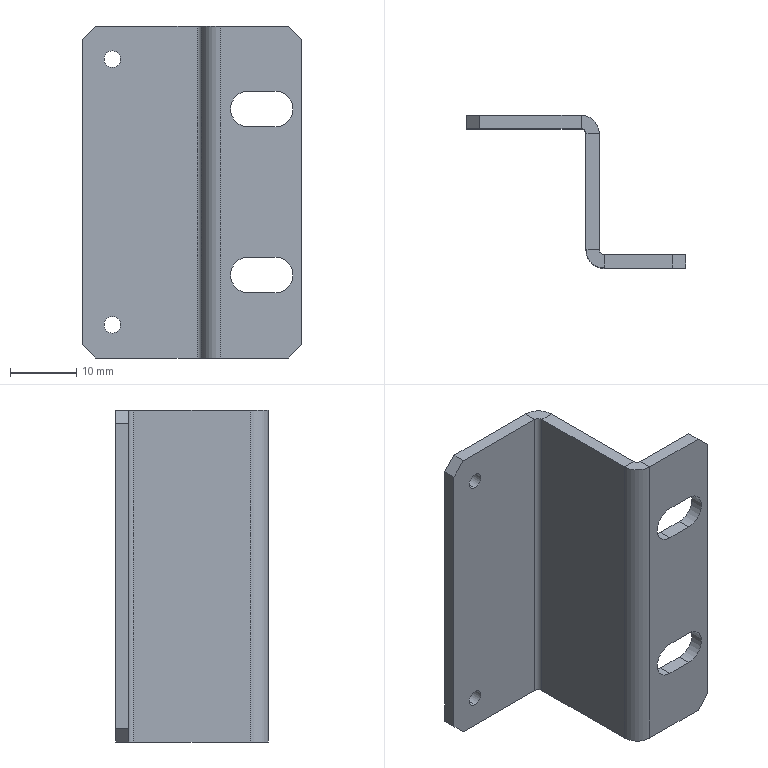Part | STEP file | 11-GYZB-JJ-00511 | 1 solid | 38 faces | box 33 x 23 x 50 mm | volume 5037 mm3 | plane 26 | cylinder 12 | commonest cylinder face diameters 2.5 x4 5.4 x4 1.473 x2 5.473 x2
STEP:
#1=CARTESIAN_POINT('',(-13.5,21.,-21.25));
#2=VERTEX_POINT('',#1);
#3=CARTESIAN_POINT('',(-13.5,21.,-18.75));
#4=VERTEX_POINT('',#3);
#5=CARTESIAN_POINT('',(-13.5,21.,-20.));
#6=DIRECTION('',(0.,1.,0.));
#7=DIRECTION('',(-1.,0.,0.));
#8=AXIS2_PLACEMENT_3D('',#5,#6,#7);
#9=CIRCLE('',#8,1.25);
#10=EDGE_CURVE('',#2,#4,#9,.T.);
#11=ORIENTED_EDGE('',*,*,#10,.F.);
#12=CARTESIAN_POINT('',(-13.5,23.,-21.25));
#13=VERTEX_POINT('',#12);
#14=CARTESIAN_POINT('',(-13.5,23.,-21.25));
#15=DIRECTION('',(0.,1.,0.));
#16=VECTOR('',#15,1000.);
#17=LINE('',#14,#16);
#18=EDGE_CURVE('',#2,#13,#17,.T.);
#19=ORIENTED_EDGE('',*,*,#18,.T.);
#20=CARTESIAN_POINT('',(-13.5,23.,-18.75));
#21=VERTEX_POINT('',#20);
#22=CARTESIAN_POINT('',(-13.5,23.,-20.));
#23=DIRECTION('',(0.,1.,0.));
#24=DIRECTION('',(0.,0.,1.));
#25=AXIS2_PLACEMENT_3D('',#22,#23,#24);
#26=CIRCLE('',#25,1.25);
#27=EDGE_CURVE('',#13,#21,#26,.T.);
#28=ORIENTED_EDGE('',*,*,#27,.T.);
#29=CARTESIAN_POINT('',(-13.5,23.,-18.75));
#30=DIRECTION('',(0.,1.,0.));
#31=VECTOR('',#30,1000.);
#32=LINE('',#29,#31);
#33=EDGE_CURVE('',#4,#21,#32,.T.);
#34=ORIENTED_EDGE('',*,*,#33,.F.);
#35=EDGE_LOOP('',(#11,#19,#28,#34));
#36=FACE_OUTER_BOUND('',#35,.T.);
#37=CARTESIAN_POINT('',(-13.5,23.,-20.));
#38=DIRECTION('',(0.,1.,0.));
#39=DIRECTION('',(0.,0.,1.));
#40=AXIS2_PLACEMENT_3D('',#37,#38,#39);
#41=CYLINDRICAL_SURFACE('',#40,1.25);
#42=ADVANCED_FACE('',(#36),#41,.F.);
#43=CARTESIAN_POINT('',(-13.5,21.,18.75));
#44=VERTEX_POINT('',#43);
#45=CARTESIAN_POINT('',(-13.5,21.,21.25));
#46=VERTEX_POINT('',#45);
#47=CARTESIAN_POINT('',(-13.5,21.,20.));
#48=DIRECTION('',(0.,1.,0.));
#49=DIRECTION('',(-1.,0.,0.));
#50=AXIS2_PLACEMENT_3D('',#47,#48,#49);
#51=CIRCLE('',#50,1.25);
#52=EDGE_CURVE('',#44,#46,#51,.T.);
#53=ORIENTED_EDGE('',*,*,#52,.F.);
#54=CARTESIAN_POINT('',(-13.5,23.,18.75));
#55=VERTEX_POINT('',#54);
#56=CARTESIAN_POINT('',(-13.5,23.,18.75));
#57=DIRECTION('',(0.,1.,0.));
#58=VECTOR('',#57,1000.);
#59=LINE('',#56,#58);
#60=EDGE_CURVE('',#44,#55,#59,.T.);
#61=ORIENTED_EDGE('',*,*,#60,.T.);
#62=CARTESIAN_POINT('',(-13.5,23.,21.25));
#63=VERTEX_POINT('',#62);
#64=CARTESIAN_POINT('',(-13.5,23.,20.));
#65=DIRECTION('',(0.,1.,0.));
#66=DIRECTION('',(0.,0.,1.));
#67=AXIS2_PLACEMENT_3D('',#64,#65,#66);
#68=CIRCLE('',#67,1.25);
#69=EDGE_CURVE('',#55,#63,#68,.T.);
#70=ORIENTED_EDGE('',*,*,#69,.T.);
#71=CARTESIAN_POINT('',(-13.5,23.,21.25));
#72=DIRECTION('',(0.,1.,0.));
#73=VECTOR('',#72,1000.);
#74=LINE('',#71,#73);
#75=EDGE_CURVE('',#46,#63,#74,.T.);
#76=ORIENTED_EDGE('',*,*,#75,.F.);
#77=EDGE_LOOP('',(#53,#61,#70,#76));
#78=FACE_OUTER_BOUND('',#77,.T.);
#79=CARTESIAN_POINT('',(-13.5,23.,20.));
#80=DIRECTION('',(0.,1.,0.));
#81=DIRECTION('',(0.,0.,1.));
#82=AXIS2_PLACEMENT_3D('',#79,#80,#81);
#83=CYLINDRICAL_SURFACE('',#82,1.25);
#84=ADVANCED_FACE('',(#78),#83,.F.);
#85=CARTESIAN_POINT('',(2.,20.263,-25.));
#86=VERTEX_POINT('',#85);
#87=CARTESIAN_POINT('',(2.,2.737,-25.));
#88=VERTEX_POINT('',#87);
#89=CARTESIAN_POINT('',(2.,0.,-25.));
#90=DIRECTION('',(0.,-1.,0.));
#91=VECTOR('',#90,1000.);
#92=LINE('',#89,#91);
#93=EDGE_CURVE('',#86,#88,#92,.T.);
#94=ORIENTED_EDGE('',*,*,#93,.F.);
#95=CARTESIAN_POINT('',(2.,20.263,25.));
#96=VERTEX_POINT('',#95);
#97=CARTESIAN_POINT('',(2.,20.263,-25.));
#98=DIRECTION('',(0.,0.,1.));
#99=VECTOR('',#98,1000.);
#100=LINE('',#97,#99);
#101=EDGE_CURVE('',#86,#96,#100,.T.);
#102=ORIENTED_EDGE('',*,*,#101,.T.);
#103=CARTESIAN_POINT('',(2.,2.737,25.));
#104=VERTEX_POINT('',#103);
#105=CARTESIAN_POINT('',(2.,0.,25.));
#106=DIRECTION('',(0.,-1.,0.));
#107=VECTOR('',#106,1000.);
#108=LINE('',#105,#107);
#109=EDGE_CURVE('',#96,#104,#108,.T.);
#110=ORIENTED_EDGE('',*,*,#109,.T.);
#111=CARTESIAN_POINT('',(2.,2.737,25.));
#112=DIRECTION('',(0.,0.,-1.));
#113=VECTOR('',#112,1000.);
#114=LINE('',#111,#113);
#115=EDGE_CURVE('',#104,#88,#114,.T.);
#116=ORIENTED_EDGE('',*,*,#115,.T.);
#117=EDGE_LOOP('',(#94,#102,#110,#116));
#118=FACE_OUTER_BOUND('',#117,.T.);
#119=CARTESIAN_POINT('',(2.,0.,25.));
#120=DIRECTION('',(1.,0.,0.));
#121=DIRECTION('',(0.,0.,-1.));
#122=AXIS2_PLACEMENT_3D('',#119,#120,#121);
#123=PLANE('',#122);
#124=ADVANCED_FACE('',(#118),#123,.T.);
#125=CARTESIAN_POINT('',(0.,20.263,-25.));
#126=VERTEX_POINT('',#125);
#127=CARTESIAN_POINT('',(0.,20.263,25.));
#128=VERTEX_POINT('',#127);
#129=CARTESIAN_POINT('',(0.,20.263,-25.));
#130=DIRECTION('',(0.,0.,1.));
#131=VECTOR('',#130,1000.);
#132=LINE('',#129,#131);
#133=EDGE_CURVE('',#126,#128,#132,.T.);
#134=ORIENTED_EDGE('',*,*,#133,.F.);
#135=CARTESIAN_POINT('',(0.,2.737,-25.));
#136=VERTEX_POINT('',#135);
#137=CARTESIAN_POINT('',(0.,0.,-25.));
#138=DIRECTION('',(0.,-1.,0.));
#139=VECTOR('',#138,1000.);
#140=LINE('',#137,#139);
#141=EDGE_CURVE('',#126,#136,#140,.T.);
#142=ORIENTED_EDGE('',*,*,#141,.T.);
#143=CARTESIAN_POINT('',(0.,2.737,25.));
#144=VERTEX_POINT('',#143);
#145=CARTESIAN_POINT('',(0.,2.737,25.));
#146=DIRECTION('',(0.,0.,-1.));
#147=VECTOR('',#146,1000.);
#148=LINE('',#145,#147);
#149=EDGE_CURVE('',#144,#136,#148,.T.);
#150=ORIENTED_EDGE('',*,*,#149,.F.);
#151=CARTESIAN_POINT('',(0.,0.,25.));
#152=DIRECTION('',(0.,-1.,0.));
#153=VECTOR('',#152,1000.);
#154=LINE('',#151,#153);
#155=EDGE_CURVE('',#128,#144,#154,.T.);
#156=ORIENTED_EDGE('',*,*,#155,.F.);
#157=EDGE_LOOP('',(#134,#142,#150,#156));
#158=FACE_OUTER_BOUND('',#157,.T.);
#159=CARTESIAN_POINT('',(0.,0.,25.));
#160=DIRECTION('',(1.,0.,0.));
#161=DIRECTION('',(0.,0.,-1.));
#162=AXIS2_PLACEMENT_3D('',#159,#160,#161);
#163=PLANE('',#162);
#164=ADVANCED_FACE('',(#158),#163,.F.);
#165=CARTESIAN_POINT('',(0.,20.263,-25.));
#166=DIRECTION('',(1.,0.,0.));
#167=VECTOR('',#166,1000.);
#168=LINE('',#165,#167);
#169=EDGE_CURVE('',#126,#86,#168,.T.);
#170=ORIENTED_EDGE('',*,*,#169,.T.);
#171=ORIENTED_EDGE('',*,*,#93,.T.);
#172=CARTESIAN_POINT('',(2.,2.737,-25.));
#173=DIRECTION('',(-1.,0.,0.));
#174=VECTOR('',#173,1000.);
#175=LINE('',#172,#174);
#176=EDGE_CURVE('',#88,#136,#175,.T.);
#177=ORIENTED_EDGE('',*,*,#176,.T.);
#178=ORIENTED_EDGE('',*,*,#141,.F.);
#179=EDGE_LOOP('',(#170,#171,#177,#178));
#180=FACE_OUTER_BOUND('',#179,.T.);
#181=CARTESIAN_POINT('',(2.737,2.737,-25.));
#182=DIRECTION('',(0.,0.,1.));
#183=DIRECTION('',(1.,0.,0.));
#184=AXIS2_PLACEMENT_3D('',#181,#182,#183);
#185=PLANE('',#184);
#186=ADVANCED_FACE('',(#180),#185,.F.);
#187=CARTESIAN_POINT('',(0.,2.737,25.));
#188=DIRECTION('',(1.,0.,0.));
#189=VECTOR('',#188,1000.);
#190=LINE('',#187,#189);
#191=EDGE_CURVE('',#144,#104,#190,.T.);
#192=ORIENTED_EDGE('',*,*,#191,.F.);
#193=CARTESIAN_POINT('',(2.737,0.,25.));
#194=VERTEX_POINT('',#193);
#195=CARTESIAN_POINT('',(2.737,2.737,25.));
#196=DIRECTION('',(0.,0.,1.));
#197=DIRECTION('',(-1.,0.,0.));
#198=AXIS2_PLACEMENT_3D('',#195,#196,#197);
#199=CIRCLE('',#198,2.737);
#200=EDGE_CURVE('',#144,#194,#199,.T.);
#201=ORIENTED_EDGE('',*,*,#200,.T.);
#202=CARTESIAN_POINT('',(2.737,2.,25.));
#203=VERTEX_POINT('',#202);
#204=CARTESIAN_POINT('',(2.737,2.,25.));
#205=DIRECTION('',(0.,-1.,0.));
#206=VECTOR('',#205,1000.);
#207=LINE('',#204,#206);
#208=EDGE_CURVE('',#203,#194,#207,.T.);
#209=ORIENTED_EDGE('',*,*,#208,.F.);
#210=CARTESIAN_POINT('',(2.737,2.737,25.));
#211=DIRECTION('',(0.,0.,1.));
#212=DIRECTION('',(1.,0.,0.));
#213=AXIS2_PLACEMENT_3D('',#210,#211,#212);
#214=CIRCLE('',#213,0.7366);
#215=EDGE_CURVE('',#104,#203,#214,.T.);
#216=ORIENTED_EDGE('',*,*,#215,.F.);
#217=EDGE_LOOP('',(#192,#201,#209,#216));
#218=FACE_OUTER_BOUND('',#217,.T.);
#219=CARTESIAN_POINT('',(0.,2.737,25.));
#220=DIRECTION('',(0.,0.,1.));
#221=DIRECTION('',(1.,0.,0.));
#222=AXIS2_PLACEMENT_3D('',#219,#220,#221);
#223=PLANE('',#222);
#224=ADVANCED_FACE('',(#218),#223,.T.);
#225=CARTESIAN_POINT('',(0.,20.263,25.));
#226=DIRECTION('',(1.,0.,0.));
#227=VECTOR('',#226,1000.);
#228=LINE('',#225,#227);
#229=EDGE_CURVE('',#128,#96,#228,.T.);
#230=ORIENTED_EDGE('',*,*,#229,.F.);
#231=ORIENTED_EDGE('',*,*,#155,.T.);
#232=ORIENTED_EDGE('',*,*,#191,.T.);
#233=ORIENTED_EDGE('',*,*,#109,.F.);
#234=EDGE_LOOP('',(#230,#231,#232,#233));
#235=FACE_OUTER_BOUND('',#234,.T.);
#236=CARTESIAN_POINT('',(2.737,2.,25.));
#237=DIRECTION('',(0.,0.,1.));
#238=DIRECTION('',(1.,0.,0.));
#239=AXIS2_PLACEMENT_3D('',#236,#237,#238);
#240=PLANE('',#239);
#241=ADVANCED_FACE('',(#235),#240,.T.);
#242=CARTESIAN_POINT('',(2.737,0.,-25.));
#243=VERTEX_POINT('',#242);
#244=CARTESIAN_POINT('',(2.737,2.,-25.));
#245=VERTEX_POINT('',#244);
#246=CARTESIAN_POINT('',(2.737,0.,-25.));
#247=DIRECTION('',(0.,1.,0.));
#248=VECTOR('',#247,1000.);
#249=LINE('',#246,#248);
#250=EDGE_CURVE('',#243,#245,#249,.T.);
#251=ORIENTED_EDGE('',*,*,#250,.F.);
#252=CARTESIAN_POINT('',(2.737,2.737,-25.));
#253=DIRECTION('',(0.,0.,1.));
#254=DIRECTION('',(-1.,0.,0.));
#255=AXIS2_PLACEMENT_3D('',#252,#253,#254);
#256=CIRCLE('',#255,2.737);
#257=EDGE_CURVE('',#136,#243,#256,.T.);
#258=ORIENTED_EDGE('',*,*,#257,.F.);
#259=ORIENTED_EDGE('',*,*,#176,.F.);
#260=CARTESIAN_POINT('',(2.737,2.737,-25.));
#261=DIRECTION('',(0.,0.,1.));
#262=DIRECTION('',(1.,0.,0.));
#263=AXIS2_PLACEMENT_3D('',#260,#261,#262);
#264=CIRCLE('',#263,0.7366);
#265=EDGE_CURVE('',#88,#245,#264,.T.);
#266=ORIENTED_EDGE('',*,*,#265,.T.);
#267=EDGE_LOOP('',(#251,#258,#259,#266));
#268=FACE_OUTER_BOUND('',#267,.T.);
#269=CARTESIAN_POINT('',(2.737,0.,-25.));
#270=DIRECTION('',(0.,0.,-1.));
#271=DIRECTION('',(-1.,0.,0.));
#272=AXIS2_PLACEMENT_3D('',#269,#270,#271);
#273=PLANE('',#272);
#274=ADVANCED_FACE('',(#268),#273,.T.);
#275=CARTESIAN_POINT('',(13.,2.,-25.));
#276=VERTEX_POINT('',#275);
#277=CARTESIAN_POINT('',(0.,2.,-25.));
#278=DIRECTION('',(1.,0.,0.));
#279=VECTOR('',#278,1000.);
#280=LINE('',#277,#279);
#281=EDGE_CURVE('',#245,#276,#280,.T.);
#282=ORIENTED_EDGE('',*,*,#281,.T.);
#283=CARTESIAN_POINT('',(13.,0.,-25.));
#284=VERTEX_POINT('',#283);
#285=CARTESIAN_POINT('',(13.,2.737,-25.));
#286=DIRECTION('',(0.,-1.,0.));
#287=VECTOR('',#286,1000.);
#288=LINE('',#285,#287);
#289=EDGE_CURVE('',#276,#284,#288,.T.);
#290=ORIENTED_EDGE('',*,*,#289,.T.);
#291=CARTESIAN_POINT('',(0.,0.,-25.));
#292=DIRECTION('',(1.,0.,0.));
#293=VECTOR('',#292,1000.);
#294=LINE('',#291,#293);
#295=EDGE_CURVE('',#243,#284,#294,.T.);
#296=ORIENTED_EDGE('',*,*,#295,.F.);
#297=ORIENTED_EDGE('',*,*,#250,.T.);
#298=EDGE_LOOP('',(#282,#290,#296,#297));
#299=FACE_OUTER_BOUND('',#298,.T.);
#300=CARTESIAN_POINT('',(2.,2.737,-25.));
#301=DIRECTION('',(0.,0.,-1.));
#302=DIRECTION('',(-1.,0.,0.));
#303=AXIS2_PLACEMENT_3D('',#300,#301,#302);
#304=PLANE('',#303);
#305=ADVANCED_FACE('',(#299),#304,.T.);
#306=CARTESIAN_POINT('',(11.,0.,-15.2));
#307=VERTEX_POINT('',#306);
#308=CARTESIAN_POINT('',(7.,0.,-15.2));
#309=VERTEX_POINT('',#308);
#310=CARTESIAN_POINT('',(7.,0.,-15.2));
#311=DIRECTION('',(-1.,0.,0.));
#312=VECTOR('',#311,1000.);
#313=LINE('',#310,#312);
#314=EDGE_CURVE('',#307,#309,#313,.T.);
#315=ORIENTED_EDGE('',*,*,#314,.T.);
#316=CARTESIAN_POINT('',(7.,0.,-9.8));
#317=VERTEX_POINT('',#316);
#318=CARTESIAN_POINT('',(7.,0.,-12.5));
#319=DIRECTION('',(0.,1.,0.));
#320=DIRECTION('',(0.,0.,-1.));
#321=AXIS2_PLACEMENT_3D('',#318,#319,#320);
#322=CIRCLE('',#321,2.7);
#323=EDGE_CURVE('',#309,#317,#322,.T.);
#324=ORIENTED_EDGE('',*,*,#323,.T.);
#325=CARTESIAN_POINT('',(11.,0.,-9.8));
#326=VERTEX_POINT('',#325);
#327=CARTESIAN_POINT('',(7.,0.,-9.8));
#328=DIRECTION('',(1.,0.,0.));
#329=VECTOR('',#328,1000.);
#330=LINE('',#327,#329);
#331=EDGE_CURVE('',#317,#326,#330,.T.);
#332=ORIENTED_EDGE('',*,*,#331,.T.);
#333=CARTESIAN_POINT('',(11.,0.,-12.5));
#334=DIRECTION('',(0.,1.,0.));
#335=DIRECTION('',(0.,0.,-1.));
#336=AXIS2_PLACEMENT_3D('',#333,#334,#335);
#337=CIRCLE('',#336,2.7);
#338=EDGE_CURVE('',#326,#307,#337,.T.);
#339=ORIENTED_EDGE('',*,*,#338,.T.);
#340=EDGE_LOOP('',(#315,#324,#332,#339));
#341=FACE_BOUND('',#340,.T.);
#342=CARTESIAN_POINT('',(11.,0.,9.8));
#343=VERTEX_POINT('',#342);
#344=CARTESIAN_POINT('',(7.,0.,9.8));
#345=VERTEX_POINT('',#344);
#346=CARTESIAN_POINT('',(7.,0.,9.8));
#347=DIRECTION('',(-1.,0.,0.));
#348=VECTOR('',#347,1000.);
#349=LINE('',#346,#348);
#350=EDGE_CURVE('',#343,#345,#349,.T.);
#351=ORIENTED_EDGE('',*,*,#350,.T.);
#352=CARTESIAN_POINT('',(7.,0.,15.2));
#353=VERTEX_POINT('',#352);
#354=CARTESIAN_POINT('',(7.,0.,12.5));
#355=DIRECTION('',(0.,1.,0.));
#356=DIRECTION('',(0.,0.,1.));
#357=AXIS2_PLACEMENT_3D('',#354,#355,#356);
#358=CIRCLE('',#357,2.7);
#359=EDGE_CURVE('',#345,#353,#358,.T.);
#360=ORIENTED_EDGE('',*,*,#359,.T.);
#361=CARTESIAN_POINT('',(11.,0.,15.2));
#362=VERTEX_POINT('',#361);
#363=CARTESIAN_POINT('',(7.,0.,15.2));
#364=DIRECTION('',(1.,0.,0.));
#365=VECTOR('',#364,1000.);
#366=LINE('',#363,#365);
#367=EDGE_CURVE('',#353,#362,#366,.T.);
#368=ORIENTED_EDGE('',*,*,#367,.T.);
#369=CARTESIAN_POINT('',(11.,0.,12.5));
#370=DIRECTION('',(0.,1.,0.));
#371=DIRECTION('',(0.,0.,1.));
#372=AXIS2_PLACEMENT_3D('',#369,#370,#371);
#373=CIRCLE('',#372,2.7);
#374=EDGE_CURVE('',#362,#343,#373,.T.);
#375=ORIENTED_EDGE('',*,*,#374,.T.);
#376=EDGE_LOOP('',(#351,#360,#368,#375));
#377=FACE_BOUND('',#376,.T.);
#378=CARTESIAN_POINT('',(15.,0.,23.));
#379=VERTEX_POINT('',#378);
#380=CARTESIAN_POINT('',(15.,0.,-23.));
#381=VERTEX_POINT('',#380);
#382=CARTESIAN_POINT('',(15.,0.,25.));
#383=DIRECTION('',(0.,0.,-1.));
#384=VECTOR('',#383,1000.);
#385=LINE('',#382,#384);
#386=EDGE_CURVE('',#379,#381,#385,.T.);
#387=ORIENTED_EDGE('',*,*,#386,.F.);
#388=CARTESIAN_POINT('',(13.,0.,25.));
#389=VERTEX_POINT('',#388);
#390=CARTESIAN_POINT('',(15.,0.,23.));
#391=DIRECTION('',(-0.7071,0.,0.7071));
#392=VECTOR('',#391,1000.);
#393=LINE('',#390,#392);
#394=EDGE_CURVE('',#379,#389,#393,.T.);
#395=ORIENTED_EDGE('',*,*,#394,.T.);
#396=CARTESIAN_POINT('',(0.,0.,25.));
#397=DIRECTION('',(1.,0.,0.));
#398=VECTOR('',#397,1000.);
#399=LINE('',#396,#398);
#400=EDGE_CURVE('',#194,#389,#399,.T.);
#401=ORIENTED_EDGE('',*,*,#400,.F.);
#402=CARTESIAN_POINT('',(2.737,0.,25.));
#403=DIRECTION('',(0.,0.,-1.));
#404=VECTOR('',#403,1000.);
#405=LINE('',#402,#404);
#406=EDGE_CURVE('',#194,#243,#405,.T.);
#407=ORIENTED_EDGE('',*,*,#406,.T.);
#408=ORIENTED_EDGE('',*,*,#295,.T.);
#409=CARTESIAN_POINT('',(13.,0.,-25.));
#410=DIRECTION('',(0.7071,0.,0.7071));
#411=VECTOR('',#410,1000.);
#412=LINE('',#409,#411);
#413=EDGE_CURVE('',#284,#381,#412,.T.);
#414=ORIENTED_EDGE('',*,*,#413,.T.);
#415=EDGE_LOOP('',(#387,#395,#401,#407,#408,#414));
#416=FACE_OUTER_BOUND('',#415,.T.);
#417=CARTESIAN_POINT('',(0.,0.,25.));
#418=DIRECTION('',(0.,1.,0.));
#419=DIRECTION('',(0.,0.,1.));
#420=AXIS2_PLACEMENT_3D('',#417,#418,#419);
#421=PLANE('',#420);
#422=ADVANCED_FACE('',(#341,#377,#416),#421,.F.);
#423=CARTESIAN_POINT('',(15.,2.,23.));
#424=VERTEX_POINT('',#423);
#425=CARTESIAN_POINT('',(15.,2.,-23.));
#426=VERTEX_POINT('',#425);
#427=CARTESIAN_POINT('',(15.,2.,25.));
#428=DIRECTION('',(0.,0.,-1.));
#429=VECTOR('',#428,1000.);
#430=LINE('',#427,#429);
#431=EDGE_CURVE('',#424,#426,#430,.T.);
#432=ORIENTED_EDGE('',*,*,#431,.F.);
#433=CARTESIAN_POINT('',(15.,2.,23.));
#434=DIRECTION('',(0.,-1.,0.));
#435=VECTOR('',#434,1000.);
#436=LINE('',#433,#435);
#437=EDGE_CURVE('',#424,#379,#436,.T.);
#438=ORIENTED_EDGE('',*,*,#437,.T.);
#439=ORIENTED_EDGE('',*,*,#386,.T.);
#440=CARTESIAN_POINT('',(15.,2.,-23.));
#441=DIRECTION('',(0.,1.,0.));
#442=VECTOR('',#441,1000.);
#443=LINE('',#440,#442);
#444=EDGE_CURVE('',#381,#426,#443,.T.);
#445=ORIENTED_EDGE('',*,*,#444,.T.);
#446=EDGE_LOOP('',(#432,#438,#439,#445));
#447=FACE_OUTER_BOUND('',#446,.T.);
#448=CARTESIAN_POINT('',(15.,2.,25.));
#449=DIRECTION('',(1.,0.,0.));
#450=DIRECTION('',(0.,0.,-1.));
#451=AXIS2_PLACEMENT_3D('',#448,#449,#450);
#452=PLANE('',#451);
#453=ADVANCED_FACE('',(#447),#452,.T.);
#454=CARTESIAN_POINT('',(7.,2.,-15.2));
#455=VERTEX_POINT('',#454);
#456=CARTESIAN_POINT('',(7.,2.,-9.8));
#457=VERTEX_POINT('',#456);
#458=CARTESIAN_POINT('',(7.,2.,-12.5));
#459=DIRECTION('',(0.,1.,0.));
#460=DIRECTION('',(0.,0.,-1.));
#461=AXIS2_PLACEMENT_3D('',#458,#459,#460);
#462=CIRCLE('',#461,2.7);
#463=EDGE_CURVE('',#455,#457,#462,.T.);
#464=ORIENTED_EDGE('',*,*,#463,.F.);
#465=CARTESIAN_POINT('',(11.,2.,-15.2));
#466=VERTEX_POINT('',#465);
#467=CARTESIAN_POINT('',(7.,2.,-15.2));
#468=DIRECTION('',(-1.,0.,0.));
#469=VECTOR('',#468,1000.);
#470=LINE('',#467,#469);
#471=EDGE_CURVE('',#466,#455,#470,.T.);
#472=ORIENTED_EDGE('',*,*,#471,.F.);
#473=CARTESIAN_POINT('',(11.,2.,-9.8));
#474=VERTEX_POINT('',#473);
#475=CARTESIAN_POINT('',(11.,2.,-12.5));
#476=DIRECTION('',(0.,1.,0.));
#477=DIRECTION('',(0.,0.,-1.));
#478=AXIS2_PLACEMENT_3D('',#475,#476,#477);
#479=CIRCLE('',#478,2.7);
#480=EDGE_CURVE('',#474,#466,#479,.T.);
#481=ORIENTED_EDGE('',*,*,#480,.F.);
#482=CARTESIAN_POINT('',(7.,2.,-9.8));
#483=DIRECTION('',(1.,0.,0.));
#484=VECTOR('',#483,1000.);
#485=LINE('',#482,#484);
#486=EDGE_CURVE('',#457,#474,#485,.T.);
#487=ORIENTED_EDGE('',*,*,#486,.F.);
#488=EDGE_LOOP('',(#464,#472,#481,#487));
#489=FACE_BOUND('',#488,.T.);
#490=CARTESIAN_POINT('',(7.,2.,9.8));
#491=VERTEX_POINT('',#490);
#492=CARTESIAN_POINT('',(7.,2.,15.2));
#493=VERTEX_POINT('',#492);
#494=CARTESIAN_POINT('',(7.,2.,12.5));
#495=DIRECTION('',(0.,1.,0.));
#496=DIRECTION('',(0.,0.,1.));
#497=AXIS2_PLACEMENT_3D('',#494,#495,#496);
#498=CIRCLE('',#497,2.7);
#499=EDGE_CURVE('',#491,#493,#498,.T.);
#500=ORIENTED_EDGE('',*,*,#499,.F.);
#501=CARTESIAN_POINT('',(11.,2.,9.8));
#502=VERTEX_POINT('',#501);
#503=CARTESIAN_POINT('',(7.,2.,9.8));
#504=DIRECTION('',(-1.,0.,0.));
#505=VECTOR('',#504,1000.);
#506=LINE('',#503,#505);
#507=EDGE_CURVE('',#502,#491,#506,.T.);
#508=ORIENTED_EDGE('',*,*,#507,.F.);
#509=CARTESIAN_POINT('',(11.,2.,15.2));
#510=VERTEX_POINT('',#509);
#511=CARTESIAN_POINT('',(11.,2.,12.5));
#512=DIRECTION('',(0.,1.,0.));
#513=DIRECTION('',(0.,0.,1.));
#514=AXIS2_PLACEMENT_3D('',#511,#512,#513);
#515=CIRCLE('',#514,2.7);
#516=EDGE_CURVE('',#510,#502,#515,.T.);
#517=ORIENTED_EDGE('',*,*,#516,.F.);
#518=CARTESIAN_POINT('',(7.,2.,15.2));
#519=DIRECTION('',(1.,0.,0.));
#520=VECTOR('',#519,1000.);
#521=LINE('',#518,#520);
#522=EDGE_CURVE('',#493,#510,#521,.T.);
#523=ORIENTED_EDGE('',*,*,#522,.F.);
#524=EDGE_LOOP('',(#500,#508,#517,#523));
#525=FACE_BOUND('',#524,.T.);
#526=CARTESIAN_POINT('',(13.,2.,25.));
#527=VERTEX_POINT('',#526);
#528=CARTESIAN_POINT('',(0.,2.,25.));
#529=DIRECTION('',(1.,0.,0.));
#530=VECTOR('',#529,1000.);
#531=LINE('',#528,#530);
#532=EDGE_CURVE('',#203,#527,#531,.T.);
#533=ORIENTED_EDGE('',*,*,#532,.T.);
#534=CARTESIAN_POINT('',(6.5,2.,31.5));
#535=DIRECTION('',(0.7071,0.,-0.7071));
#536=VECTOR('',#535,1000.);
#537=LINE('',#534,#536);
#538=EDGE_CURVE('',#527,#424,#537,.T.);
#539=ORIENTED_EDGE('',*,*,#538,.T.);
#540=ORIENTED_EDGE('',*,*,#431,.T.);
#541=CARTESIAN_POINT('',(31.5,2.,-6.5));
#542=DIRECTION('',(-0.7071,0.,-0.7071));
#543=VECTOR('',#542,1000.);
#544=LINE('',#541,#543);
#545=EDGE_CURVE('',#426,#276,#544,.T.);
#546=ORIENTED_EDGE('',*,*,#545,.T.);
#547=ORIENTED_EDGE('',*,*,#281,.F.);
#548=CARTESIAN_POINT('',(2.737,2.,25.));
#549=DIRECTION('',(0.,0.,-1.));
#550=VECTOR('',#549,1000.);
#551=LINE('',#548,#550);
#552=EDGE_CURVE('',#203,#245,#551,.T.);
#553=ORIENTED_EDGE('',*,*,#552,.F.);
#554=EDGE_LOOP('',(#533,#539,#540,#546,#547,#553));
#555=FACE_OUTER_BOUND('',#554,.T.);
#556=CARTESIAN_POINT('',(0.,2.,25.));
#557=DIRECTION('',(0.,1.,0.));
#558=DIRECTION('',(0.,0.,1.));
#559=AXIS2_PLACEMENT_3D('',#556,#557,#558);
#560=PLANE('',#559);
#561=ADVANCED_FACE('',(#489,#525,#555),#560,.T.);
#562=ORIENTED_EDGE('',*,*,#265,.F.);
#563=ORIENTED_EDGE('',*,*,#115,.F.);
#564=ORIENTED_EDGE('',*,*,#215,.T.);
#565=ORIENTED_EDGE('',*,*,#552,.T.);
#566=EDGE_LOOP('',(#562,#563,#564,#565));
#567=FACE_OUTER_BOUND('',#566,.T.);
#568=CARTESIAN_POINT('',(2.737,2.737,25.));
#569=DIRECTION('',(0.,0.,-1.));
#570=DIRECTION('',(-1.,0.,0.));
#571=AXIS2_PLACEMENT_3D('',#568,#569,#570);
#572=CYLINDRICAL_SURFACE('',#571,0.7366);
#573=ADVANCED_FACE('',(#567),#572,.F.);
#574=ORIENTED_EDGE('',*,*,#257,.T.);
#575=ORIENTED_EDGE('',*,*,#406,.F.);
#576=ORIENTED_EDGE('',*,*,#200,.F.);
#577=ORIENTED_EDGE('',*,*,#149,.T.);
#578=EDGE_LOOP('',(#574,#575,#576,#577));
#579=FACE_OUTER_BOUND('',#578,.T.);
#580=CARTESIAN_POINT('',(2.737,2.737,25.));
#581=DIRECTION('',(0.,0.,-1.));
#582=DIRECTION('',(-1.,0.,0.));
#583=AXIS2_PLACEMENT_3D('',#580,#581,#582);
#584=CYLINDRICAL_SURFACE('',#583,2.737);
#585=ADVANCED_FACE('',(#579),#584,.T.);
#586=ORIENTED_EDGE('',*,*,#400,.T.);
#587=CARTESIAN_POINT('',(13.,2.737,25.));
#588=DIRECTION('',(0.,1.,0.));
#589=VECTOR('',#588,1000.);
#590=LINE('',#587,#589);
#591=EDGE_CURVE('',#389,#527,#590,.T.);
#592=ORIENTED_EDGE('',*,*,#591,.T.);
#593=ORIENTED_EDGE('',*,*,#532,.F.);
#594=ORIENTED_EDGE('',*,*,#208,.T.);
#595=EDGE_LOOP('',(#586,#592,#593,#594));
#596=FACE_OUTER_BOUND('',#595,.T.);
#597=CARTESIAN_POINT('',(2.737,2.737,25.));
#598=DIRECTION('',(0.,0.,1.));
#599=DIRECTION('',(1.,0.,0.));
#600=AXIS2_PLACEMENT_3D('',#597,#598,#599);
#601=PLANE('',#600);
#602=ADVANCED_FACE('',(#596),#601,.T.);
#603=ORIENTED_EDGE('',*,*,#499,.T.);
#604=CARTESIAN_POINT('',(7.,0.,15.2));
#605=DIRECTION('',(0.,1.,0.));
#606=VECTOR('',#605,1000.);
#607=LINE('',#604,#606);
#608=EDGE_CURVE('',#353,#493,#607,.T.);
#609=ORIENTED_EDGE('',*,*,#608,.F.);
#610=ORIENTED_EDGE('',*,*,#359,.F.);
#611=CARTESIAN_POINT('',(7.,0.,9.8));
#612=DIRECTION('',(0.,1.,0.));
#613=VECTOR('',#612,1000.);
#614=LINE('',#611,#613);
#615=EDGE_CURVE('',#345,#491,#614,.T.);
#616=ORIENTED_EDGE('',*,*,#615,.T.);
#617=EDGE_LOOP('',(#603,#609,#610,#616));
#618=FACE_OUTER_BOUND('',#617,.T.);
#619=CARTESIAN_POINT('',(7.,0.,12.5));
#620=DIRECTION('',(0.,1.,0.));
#621=DIRECTION('',(0.,0.,1.));
#622=AXIS2_PLACEMENT_3D('',#619,#620,#621);
#623=CYLINDRICAL_SURFACE('',#622,2.7);
#624=ADVANCED_FACE('',(#618),#623,.F.);
#625=ORIENTED_EDGE('',*,*,#507,.T.);
#626=ORIENTED_EDGE('',*,*,#615,.F.);
#627=ORIENTED_EDGE('',*,*,#350,.F.);
#628=CARTESIAN_POINT('',(11.,0.,9.8));
#629=DIRECTION('',(0.,1.,0.));
#630=VECTOR('',#629,1000.);
#631=LINE('',#628,#630);
#632=EDGE_CURVE('',#343,#502,#631,.T.);
#633=ORIENTED_EDGE('',*,*,#632,.T.);
#634=EDGE_LOOP('',(#625,#626,#627,#633));
#635=FACE_OUTER_BOUND('',#634,.T.);
#636=CARTESIAN_POINT('',(7.,0.,9.8));
#637=DIRECTION('',(0.,0.,-1.));
#638=DIRECTION('',(-1.,0.,0.));
#639=AXIS2_PLACEMENT_3D('',#636,#637,#638);
#640=PLANE('',#639);
#641=ADVANCED_FACE('',(#635),#640,.F.);
#642=ORIENTED_EDGE('',*,*,#516,.T.);
#643=ORIENTED_EDGE('',*,*,#632,.F.);
#644=ORIENTED_EDGE('',*,*,#374,.F.);
#645=CARTESIAN_POINT('',(11.,0.,15.2));
#646=DIRECTION('',(0.,1.,0.));
#647=VECTOR('',#646,1000.);
#648=LINE('',#645,#647);
#649=EDGE_CURVE('',#362,#510,#648,.T.);
#650=ORIENTED_EDGE('',*,*,#649,.T.);
#651=EDGE_LOOP('',(#642,#643,#644,#650));
#652=FACE_OUTER_BOUND('',#651,.T.);
#653=CARTESIAN_POINT('',(11.,0.,12.5));
#654=DIRECTION('',(0.,1.,0.));
#655=DIRECTION('',(0.,0.,1.));
#656=AXIS2_PLACEMENT_3D('',#653,#654,#655);
#657=CYLINDRICAL_SURFACE('',#656,2.7);
#658=ADVANCED_FACE('',(#652),#657,.F.);
#659=ORIENTED_EDGE('',*,*,#522,.T.);
#660=ORIENTED_EDGE('',*,*,#649,.F.);
#661=ORIENTED_EDGE('',*,*,#367,.F.);
#662=ORIENTED_EDGE('',*,*,#608,.T.);
#663=EDGE_LOOP('',(#659,#660,#661,#662));
#664=FACE_OUTER_BOUND('',#663,.T.);
#665=CARTESIAN_POINT('',(7.,0.,15.2));
#666=DIRECTION('',(0.,0.,1.));
#667=DIRECTION('',(1.,0.,0.));
#668=AXIS2_PLACEMENT_3D('',#665,#666,#667);
#669=PLANE('',#668);
#670=ADVANCED_FACE('',(#664),#669,.F.);
#671=ORIENTED_EDGE('',*,*,#463,.T.);
#672=CARTESIAN_POINT('',(7.,0.,-9.8));
#673=DIRECTION('',(0.,1.,0.));
#674=VECTOR('',#673,1000.);
#675=LINE('',#672,#674);
#676=EDGE_CURVE('',#317,#457,#675,.T.);
#677=ORIENTED_EDGE('',*,*,#676,.F.);
#678=ORIENTED_EDGE('',*,*,#323,.F.);
#679=CARTESIAN_POINT('',(7.,0.,-15.2));
#680=DIRECTION('',(0.,1.,0.));
#681=VECTOR('',#680,1000.);
#682=LINE('',#679,#681);
#683=EDGE_CURVE('',#309,#455,#682,.T.);
#684=ORIENTED_EDGE('',*,*,#683,.T.);
#685=EDGE_LOOP('',(#671,#677,#678,#684));
#686=FACE_OUTER_BOUND('',#685,.T.);
#687=CARTESIAN_POINT('',(7.,0.,-12.5));
#688=DIRECTION('',(0.,1.,0.));
#689=DIRECTION('',(0.,0.,1.));
#690=AXIS2_PLACEMENT_3D('',#687,#688,#689);
#691=CYLINDRICAL_SURFACE('',#690,2.7);
#692=ADVANCED_FACE('',(#686),#691,.F.);
#693=ORIENTED_EDGE('',*,*,#471,.T.);
#694=ORIENTED_EDGE('',*,*,#683,.F.);
#695=ORIENTED_EDGE('',*,*,#314,.F.);
#696=CARTESIAN_POINT('',(11.,0.,-15.2));
#697=DIRECTION('',(0.,1.,0.));
#698=VECTOR('',#697,1000.);
#699=LINE('',#696,#698);
#700=EDGE_CURVE('',#307,#466,#699,.T.);
#701=ORIENTED_EDGE('',*,*,#700,.T.);
#702=EDGE_LOOP('',(#693,#694,#695,#701));
#703=FACE_OUTER_BOUND('',#702,.T.);
#704=CARTESIAN_POINT('',(7.,0.,-15.2));
#705=DIRECTION('',(0.,0.,-1.));
#706=DIRECTION('',(-1.,0.,0.));
#707=AXIS2_PLACEMENT_3D('',#704,#705,#706);
#708=PLANE('',#707);
#709=ADVANCED_FACE('',(#703),#708,.F.);
#710=ORIENTED_EDGE('',*,*,#480,.T.);
#711=ORIENTED_EDGE('',*,*,#700,.F.);
#712=ORIENTED_EDGE('',*,*,#338,.F.);
#713=CARTESIAN_POINT('',(11.,0.,-9.8));
#714=DIRECTION('',(0.,1.,0.));
#715=VECTOR('',#714,1000.);
#716=LINE('',#713,#715);
#717=EDGE_CURVE('',#326,#474,#716,.T.);
#718=ORIENTED_EDGE('',*,*,#717,.T.);
#719=EDGE_LOOP('',(#710,#711,#712,#718));
#720=FACE_OUTER_BOUND('',#719,.T.);
#721=CARTESIAN_POINT('',(11.,0.,-12.5));
#722=DIRECTION('',(0.,1.,0.));
#723=DIRECTION('',(0.,0.,1.));
#724=AXIS2_PLACEMENT_3D('',#721,#722,#723);
#725=CYLINDRICAL_SURFACE('',#724,2.7);
#726=ADVANCED_FACE('',(#720),#725,.F.);
#727=ORIENTED_EDGE('',*,*,#486,.T.);
#728=ORIENTED_EDGE('',*,*,#717,.F.);
#729=ORIENTED_EDGE('',*,*,#331,.F.);
#730=ORIENTED_EDGE('',*,*,#676,.T.);
#731=EDGE_LOOP('',(#727,#728,#729,#730));
#732=FACE_OUTER_BOUND('',#731,.T.);
#733=CARTESIAN_POINT('',(7.,0.,-9.8));
#734=DIRECTION('',(0.,0.,1.));
#735=DIRECTION('',(1.,0.,0.));
#736=AXIS2_PLACEMENT_3D('',#733,#734,#735);
#737=PLANE('',#736);
#738=ADVANCED_FACE('',(#732),#737,.F.);
#739=CARTESIAN_POINT('',(-0.7366,21.,25.));
#740=VERTEX_POINT('',#739);
#741=CARTESIAN_POINT('',(-0.7366,23.,25.));
#742=VERTEX_POINT('',#741);
#743=CARTESIAN_POINT('',(-0.7366,23.,25.));
#744=DIRECTION('',(0.,1.,0.));
#745=VECTOR('',#744,1000.);
#746=LINE('',#743,#745);
#747=EDGE_CURVE('',#740,#742,#746,.T.);
#748=ORIENTED_EDGE('',*,*,#747,.F.);
#749=CARTESIAN_POINT('',(-0.7366,20.263,25.));
#750=DIRECTION('',(0.,0.,1.));
#751=DIRECTION('',(-1.,0.,0.));
#752=AXIS2_PLACEMENT_3D('',#749,#750,#751);
#753=CIRCLE('',#752,0.7366);
#754=EDGE_CURVE('',#128,#740,#753,.T.);
#755=ORIENTED_EDGE('',*,*,#754,.F.);
#756=ORIENTED_EDGE('',*,*,#229,.T.);
#757=CARTESIAN_POINT('',(-0.7366,20.263,25.));
#758=DIRECTION('',(0.,0.,1.));
#759=DIRECTION('',(-1.,0.,0.));
#760=AXIS2_PLACEMENT_3D('',#757,#758,#759);
#761=CIRCLE('',#760,2.737);
#762=EDGE_CURVE('',#96,#742,#761,.T.);
#763=ORIENTED_EDGE('',*,*,#762,.T.);
#764=EDGE_LOOP('',(#748,#755,#756,#763));
#765=FACE_OUTER_BOUND('',#764,.T.);
#766=CARTESIAN_POINT('',(-0.7366,20.263,25.));
#767=DIRECTION('',(0.,0.,1.));
#768=DIRECTION('',(1.,0.,0.));
#769=AXIS2_PLACEMENT_3D('',#766,#767,#768);
#770=PLANE('',#769);
#771=ADVANCED_FACE('',(#765),#770,.T.);
#772=CARTESIAN_POINT('',(-0.7366,21.,-25.));
#773=VERTEX_POINT('',#772);
#774=CARTESIAN_POINT('',(-0.7366,20.263,-25.));
#775=DIRECTION('',(0.,0.,-1.));
#776=DIRECTION('',(-1.,0.,0.));
#777=AXIS2_PLACEMENT_3D('',#774,#775,#776);
#778=CIRCLE('',#777,0.7366);
#779=EDGE_CURVE('',#773,#126,#778,.T.);
#780=ORIENTED_EDGE('',*,*,#779,.F.);
#781=CARTESIAN_POINT('',(-0.7366,23.,-25.));
#782=VERTEX_POINT('',#781);
#783=CARTESIAN_POINT('',(-0.7366,21.,-25.));
#784=DIRECTION('',(0.,1.,0.));
#785=VECTOR('',#784,1000.);
#786=LINE('',#783,#785);
#787=EDGE_CURVE('',#773,#782,#786,.T.);
#788=ORIENTED_EDGE('',*,*,#787,.T.);
#789=CARTESIAN_POINT('',(-0.7366,20.263,-25.));
#790=DIRECTION('',(0.,0.,-1.));
#791=DIRECTION('',(-1.,0.,0.));
#792=AXIS2_PLACEMENT_3D('',#789,#790,#791);
#793=CIRCLE('',#792,2.737);
#794=EDGE_CURVE('',#782,#86,#793,.T.);
#795=ORIENTED_EDGE('',*,*,#794,.T.);
#796=ORIENTED_EDGE('',*,*,#169,.F.);
#797=EDGE_LOOP('',(#780,#788,#795,#796));
#798=FACE_OUTER_BOUND('',#797,.T.);
#799=CARTESIAN_POINT('',(-0.7366,20.263,-25.));
#800=DIRECTION('',(0.,0.,1.));
#801=DIRECTION('',(1.,0.,0.));
#802=AXIS2_PLACEMENT_3D('',#799,#800,#801);
#803=PLANE('',#802);
#804=ADVANCED_FACE('',(#798),#803,.F.);
#805=ORIENTED_EDGE('',*,*,#101,.F.);
#806=ORIENTED_EDGE('',*,*,#794,.F.);
#807=CARTESIAN_POINT('',(-0.7366,23.,0.));
#808=DIRECTION('',(0.,0.,-1.));
#809=VECTOR('',#808,1000.);
#810=LINE('',#807,#809);
#811=EDGE_CURVE('',#742,#782,#810,.T.);
#812=ORIENTED_EDGE('',*,*,#811,.F.);
#813=ORIENTED_EDGE('',*,*,#762,.F.);
#814=EDGE_LOOP('',(#805,#806,#812,#813));
#815=FACE_OUTER_BOUND('',#814,.T.);
#816=CARTESIAN_POINT('',(-0.7366,20.263,-25.));
#817=DIRECTION('',(0.,0.,-1.));
#818=DIRECTION('',(0.,1.,0.));
#819=AXIS2_PLACEMENT_3D('',#816,#817,#818);
#820=CYLINDRICAL_SURFACE('',#819,2.737);
#821=ADVANCED_FACE('',(#815),#820,.T.);
#822=ORIENTED_EDGE('',*,*,#133,.T.);
#823=ORIENTED_EDGE('',*,*,#754,.T.);
#824=CARTESIAN_POINT('',(-0.7366,21.,25.));
#825=DIRECTION('',(0.,0.,-1.));
#826=VECTOR('',#825,1000.);
#827=LINE('',#824,#826);
#828=EDGE_CURVE('',#740,#773,#827,.T.);
#829=ORIENTED_EDGE('',*,*,#828,.T.);
#830=ORIENTED_EDGE('',*,*,#779,.T.);
#831=EDGE_LOOP('',(#822,#823,#829,#830));
#832=FACE_OUTER_BOUND('',#831,.T.);
#833=CARTESIAN_POINT('',(-0.7366,20.263,-25.));
#834=DIRECTION('',(0.,0.,-1.));
#835=DIRECTION('',(0.,1.,0.));
#836=AXIS2_PLACEMENT_3D('',#833,#834,#835);
#837=CYLINDRICAL_SURFACE('',#836,0.7366);
#838=ADVANCED_FACE('',(#832),#837,.F.);
#839=CARTESIAN_POINT('',(-16.,21.,-25.));
#840=VERTEX_POINT('',#839);
#841=CARTESIAN_POINT('',(0.,21.,-25.));
#842=DIRECTION('',(1.,0.,0.));
#843=VECTOR('',#842,1000.);
#844=LINE('',#841,#843);
#845=EDGE_CURVE('',#840,#773,#844,.T.);
#846=ORIENTED_EDGE('',*,*,#845,.F.);
#847=CARTESIAN_POINT('',(-16.,23.,-25.));
#848=VERTEX_POINT('',#847);
#849=CARTESIAN_POINT('',(-16.,23.,-25.));
#850=DIRECTION('',(0.,1.,0.));
#851=VECTOR('',#850,1000.);
#852=LINE('',#849,#851);
#853=EDGE_CURVE('',#840,#848,#852,.T.);
#854=ORIENTED_EDGE('',*,*,#853,.T.);
#855=CARTESIAN_POINT('',(0.,23.,-25.));
#856=DIRECTION('',(1.,0.,0.));
#857=VECTOR('',#856,1000.);
#858=LINE('',#855,#857);
#859=EDGE_CURVE('',#848,#782,#858,.T.);
#860=ORIENTED_EDGE('',*,*,#859,.T.);
#861=ORIENTED_EDGE('',*,*,#787,.F.);
#862=EDGE_LOOP('',(#846,#854,#860,#861));
#863=FACE_OUTER_BOUND('',#862,.T.);
#864=CARTESIAN_POINT('',(0.,23.,-25.));
#865=DIRECTION('',(0.,0.,-1.));
#866=DIRECTION('',(-1.,0.,0.));
#867=AXIS2_PLACEMENT_3D('',#864,#865,#866);
#868=PLANE('',#867);
#869=ADVANCED_FACE('',(#863),#868,.T.);
#870=CARTESIAN_POINT('',(-16.,23.,25.));
#871=VERTEX_POINT('',#870);
#872=CARTESIAN_POINT('',(-18.,23.,25.));
#873=DIRECTION('',(-1.,0.,0.));
#874=VECTOR('',#873,1000.);
#875=LINE('',#872,#874);
#876=EDGE_CURVE('',#742,#871,#875,.T.);
#877=ORIENTED_EDGE('',*,*,#876,.T.);
#878=CARTESIAN_POINT('',(-16.,21.,25.));
#879=VERTEX_POINT('',#878);
#880=CARTESIAN_POINT('',(-16.,23.,25.));
#881=DIRECTION('',(0.,-1.,0.));
#882=VECTOR('',#881,1000.);
#883=LINE('',#880,#882);
#884=EDGE_CURVE('',#871,#879,#883,.T.);
#885=ORIENTED_EDGE('',*,*,#884,.T.);
#886=CARTESIAN_POINT('',(0.,21.,25.));
#887=DIRECTION('',(-1.,0.,0.));
#888=VECTOR('',#887,1000.);
#889=LINE('',#886,#888);
#890=EDGE_CURVE('',#740,#879,#889,.T.);
#891=ORIENTED_EDGE('',*,*,#890,.F.);
#892=ORIENTED_EDGE('',*,*,#747,.T.);
#893=EDGE_LOOP('',(#877,#885,#891,#892));
#894=FACE_OUTER_BOUND('',#893,.T.);
#895=CARTESIAN_POINT('',(-18.,23.,25.));
#896=DIRECTION('',(0.,0.,1.));
#897=DIRECTION('',(1.,0.,0.));
#898=AXIS2_PLACEMENT_3D('',#895,#896,#897);
#899=PLANE('',#898);
#900=ADVANCED_FACE('',(#894),#899,.T.);
#901=CARTESIAN_POINT('',(-13.5,23.,-20.));
#902=DIRECTION('',(0.,1.,0.));
#903=DIRECTION('',(0.,0.,1.));
#904=AXIS2_PLACEMENT_3D('',#901,#902,#903);
#905=CIRCLE('',#904,1.25);
#906=EDGE_CURVE('',#21,#13,#905,.T.);
#907=ORIENTED_EDGE('',*,*,#906,.F.);
#908=ORIENTED_EDGE('',*,*,#27,.F.);
#909=EDGE_LOOP('',(#907,#908));
#910=FACE_BOUND('',#909,.T.);
#911=CARTESIAN_POINT('',(-13.5,23.,20.));
#912=DIRECTION('',(0.,1.,0.));
#913=DIRECTION('',(0.,0.,1.));
#914=AXIS2_PLACEMENT_3D('',#911,#912,#913);
#915=CIRCLE('',#914,1.25);
#916=EDGE_CURVE('',#63,#55,#915,.T.);
#917=ORIENTED_EDGE('',*,*,#916,.F.);
#918=ORIENTED_EDGE('',*,*,#69,.F.);
#919=EDGE_LOOP('',(#917,#918));
#920=FACE_BOUND('',#919,.T.);
#921=ORIENTED_EDGE('',*,*,#859,.F.);
#922=CARTESIAN_POINT('',(-18.,23.,-23.));
#923=VERTEX_POINT('',#922);
#924=CARTESIAN_POINT('',(-20.5,23.,-20.5));
#925=DIRECTION('',(-0.7071,0.,0.7071));
#926=VECTOR('',#925,1000.);
#927=LINE('',#924,#926);
#928=EDGE_CURVE('',#848,#923,#927,.T.);
#929=ORIENTED_EDGE('',*,*,#928,.T.);
#930=CARTESIAN_POINT('',(-18.,23.,23.));
#931=VERTEX_POINT('',#930);
#932=CARTESIAN_POINT('',(-18.,23.,-25.));
#933=DIRECTION('',(0.,0.,-1.));
#934=VECTOR('',#933,1000.);
#935=LINE('',#932,#934);
#936=EDGE_CURVE('',#931,#923,#935,.T.);
#937=ORIENTED_EDGE('',*,*,#936,.F.);
#938=CARTESIAN_POINT('',(-20.5,23.,20.5));
#939=DIRECTION('',(0.7071,0.,0.7071));
#940=VECTOR('',#939,1000.);
#941=LINE('',#938,#940);
#942=EDGE_CURVE('',#931,#871,#941,.T.);
#943=ORIENTED_EDGE('',*,*,#942,.T.);
#944=ORIENTED_EDGE('',*,*,#876,.F.);
#945=ORIENTED_EDGE('',*,*,#811,.T.);
#946=EDGE_LOOP('',(#921,#929,#937,#943,#944,#945));
#947=FACE_OUTER_BOUND('',#946,.T.);
#948=CARTESIAN_POINT('',(0.,23.,0.));
#949=DIRECTION('',(0.,1.,0.));
#950=DIRECTION('',(-1.,0.,0.));
#951=AXIS2_PLACEMENT_3D('',#948,#949,#950);
#952=PLANE('',#951);
#953=ADVANCED_FACE('',(#910,#920,#947),#952,.T.);
#954=CARTESIAN_POINT('',(-13.5,21.,-20.));
#955=DIRECTION('',(0.,1.,0.));
#956=DIRECTION('',(-1.,0.,0.));
#957=AXIS2_PLACEMENT_3D('',#954,#955,#956);
#958=CIRCLE('',#957,1.25);
#959=EDGE_CURVE('',#4,#2,#958,.T.);
#960=ORIENTED_EDGE('',*,*,#959,.T.);
#961=ORIENTED_EDGE('',*,*,#10,.T.);
#962=EDGE_LOOP('',(#960,#961));
#963=FACE_BOUND('',#962,.T.);
#964=CARTESIAN_POINT('',(-13.5,21.,20.));
#965=DIRECTION('',(0.,1.,0.));
#966=DIRECTION('',(-1.,0.,0.));
#967=AXIS2_PLACEMENT_3D('',#964,#965,#966);
#968=CIRCLE('',#967,1.25);
#969=EDGE_CURVE('',#46,#44,#968,.T.);
#970=ORIENTED_EDGE('',*,*,#969,.T.);
#971=ORIENTED_EDGE('',*,*,#52,.T.);
#972=EDGE_LOOP('',(#970,#971));
#973=FACE_BOUND('',#972,.T.);
#974=CARTESIAN_POINT('',(-18.,21.,23.));
#975=VERTEX_POINT('',#974);
#976=CARTESIAN_POINT('',(-18.,21.,-23.));
#977=VERTEX_POINT('',#976);
#978=CARTESIAN_POINT('',(-18.,21.,0.));
#979=DIRECTION('',(0.,0.,-1.));
#980=VECTOR('',#979,1000.);
#981=LINE('',#978,#980);
#982=EDGE_CURVE('',#975,#977,#981,.T.);
#983=ORIENTED_EDGE('',*,*,#982,.T.);
#984=CARTESIAN_POINT('',(-18.,21.,-23.));
#985=DIRECTION('',(0.7071,0.,-0.7071));
#986=VECTOR('',#985,1000.);
#987=LINE('',#984,#986);
#988=EDGE_CURVE('',#977,#840,#987,.T.);
#989=ORIENTED_EDGE('',*,*,#988,.T.);
#990=ORIENTED_EDGE('',*,*,#845,.T.);
#991=ORIENTED_EDGE('',*,*,#828,.F.);
#992=ORIENTED_EDGE('',*,*,#890,.T.);
#993=CARTESIAN_POINT('',(-16.,21.,25.));
#994=DIRECTION('',(-0.7071,0.,-0.7071));
#995=VECTOR('',#994,1000.);
#996=LINE('',#993,#995);
#997=EDGE_CURVE('',#879,#975,#996,.T.);
#998=ORIENTED_EDGE('',*,*,#997,.T.);
#999=EDGE_LOOP('',(#983,#989,#990,#991,#992,#998));
#1000=FACE_OUTER_BOUND('',#999,.T.);
#1001=CARTESIAN_POINT('',(0.,21.,0.));
#1002=DIRECTION('',(0.,1.,0.));
#1003=DIRECTION('',(-1.,0.,0.));
#1004=AXIS2_PLACEMENT_3D('',#1001,#1002,#1003);
#1005=PLANE('',#1004);
#1006=ADVANCED_FACE('',(#963,#973,#1000),#1005,.F.);
#1007=ORIENTED_EDGE('',*,*,#936,.T.);
#1008=CARTESIAN_POINT('',(-18.,23.,-23.));
#1009=DIRECTION('',(0.,-1.,0.));
#1010=VECTOR('',#1009,1000.);
#1011=LINE('',#1008,#1010);
#1012=EDGE_CURVE('',#923,#977,#1011,.T.);
#1013=ORIENTED_EDGE('',*,*,#1012,.T.);
#1014=ORIENTED_EDGE('',*,*,#982,.F.);
#1015=CARTESIAN_POINT('',(-18.,23.,23.));
#1016=DIRECTION('',(0.,1.,0.));
#1017=VECTOR('',#1016,1000.);
#1018=LINE('',#1015,#1017);
#1019=EDGE_CURVE('',#975,#931,#1018,.T.);
#1020=ORIENTED_EDGE('',*,*,#1019,.T.);
#1021=EDGE_LOOP('',(#1007,#1013,#1014,#1020));
#1022=FACE_OUTER_BOUND('',#1021,.T.);
#1023=CARTESIAN_POINT('',(-18.,23.,-25.));
#1024=DIRECTION('',(-1.,0.,0.));
#1025=DIRECTION('',(0.,-1.,0.));
#1026=AXIS2_PLACEMENT_3D('',#1023,#1024,#1025);
#1027=PLANE('',#1026);
#1028=ADVANCED_FACE('',(#1022),#1027,.T.);
#1029=ORIENTED_EDGE('',*,*,#60,.F.);
#1030=ORIENTED_EDGE('',*,*,#969,.F.);
#1031=ORIENTED_EDGE('',*,*,#75,.T.);
#1032=ORIENTED_EDGE('',*,*,#916,.T.);
#1033=EDGE_LOOP('',(#1029,#1030,#1031,#1032));
#1034=FACE_OUTER_BOUND('',#1033,.T.);
#1035=CARTESIAN_POINT('',(-13.5,23.,20.));
#1036=DIRECTION('',(0.,1.,0.));
#1037=DIRECTION('',(0.,0.,1.));
#1038=AXIS2_PLACEMENT_3D('',#1035,#1036,#1037);
#1039=CYLINDRICAL_SURFACE('',#1038,1.25);
#1040=ADVANCED_FACE('',(#1034),#1039,.F.);
#1041=ORIENTED_EDGE('',*,*,#18,.F.);
#1042=ORIENTED_EDGE('',*,*,#959,.F.);
#1043=ORIENTED_EDGE('',*,*,#33,.T.);
#1044=ORIENTED_EDGE('',*,*,#906,.T.);
#1045=EDGE_LOOP('',(#1041,#1042,#1043,#1044));
#1046=FACE_OUTER_BOUND('',#1045,.T.);
#1047=CARTESIAN_POINT('',(-13.5,23.,-20.));
#1048=DIRECTION('',(0.,1.,0.));
#1049=DIRECTION('',(0.,0.,1.));
#1050=AXIS2_PLACEMENT_3D('',#1047,#1048,#1049);
#1051=CYLINDRICAL_SURFACE('',#1050,1.25);
#1052=ADVANCED_FACE('',(#1046),#1051,.F.);
#1053=ORIENTED_EDGE('',*,*,#928,.F.);
#1054=ORIENTED_EDGE('',*,*,#853,.F.);
#1055=ORIENTED_EDGE('',*,*,#988,.F.);
#1056=ORIENTED_EDGE('',*,*,#1012,.F.);
#1057=EDGE_LOOP('',(#1053,#1054,#1055,#1056));
#1058=FACE_OUTER_BOUND('',#1057,.T.);
#1059=CARTESIAN_POINT('',(-18.,23.,-23.));
#1060=DIRECTION('',(0.7071,0.,0.7071));
#1061=DIRECTION('',(0.,-1.,0.));
#1062=AXIS2_PLACEMENT_3D('',#1059,#1060,#1061);
#1063=PLANE('',#1062);
#1064=ADVANCED_FACE('',(#1058),#1063,.F.);
#1065=ORIENTED_EDGE('',*,*,#942,.F.);
#1066=ORIENTED_EDGE('',*,*,#1019,.F.);
#1067=ORIENTED_EDGE('',*,*,#997,.F.);
#1068=ORIENTED_EDGE('',*,*,#884,.F.);
#1069=EDGE_LOOP('',(#1065,#1066,#1067,#1068));
#1070=FACE_OUTER_BOUND('',#1069,.T.);
#1071=CARTESIAN_POINT('',(-16.,23.,25.));
#1072=DIRECTION('',(0.7071,0.,-0.7071));
#1073=DIRECTION('',(0.,-1.,0.));
#1074=AXIS2_PLACEMENT_3D('',#1071,#1072,#1073);
#1075=PLANE('',#1074);
#1076=ADVANCED_FACE('',(#1070),#1075,.F.);
#1077=ORIENTED_EDGE('',*,*,#538,.F.);
#1078=ORIENTED_EDGE('',*,*,#591,.F.);
#1079=ORIENTED_EDGE('',*,*,#394,.F.);
#1080=ORIENTED_EDGE('',*,*,#437,.F.);
#1081=EDGE_LOOP('',(#1077,#1078,#1079,#1080));
#1082=FACE_OUTER_BOUND('',#1081,.T.);
#1083=CARTESIAN_POINT('',(15.,2.,23.));
#1084=DIRECTION('',(-0.7071,0.,-0.7071));
#1085=DIRECTION('',(0.,-1.,0.));
#1086=AXIS2_PLACEMENT_3D('',#1083,#1084,#1085);
#1087=PLANE('',#1086);
#1088=ADVANCED_FACE('',(#1082),#1087,.F.);
#1089=ORIENTED_EDGE('',*,*,#545,.F.);
#1090=ORIENTED_EDGE('',*,*,#444,.F.);
#1091=ORIENTED_EDGE('',*,*,#413,.F.);
#1092=ORIENTED_EDGE('',*,*,#289,.F.);
#1093=EDGE_LOOP('',(#1089,#1090,#1091,#1092));
#1094=FACE_OUTER_BOUND('',#1093,.T.);
#1095=CARTESIAN_POINT('',(13.,2.737,-25.));
#1096=DIRECTION('',(-0.7071,0.,0.7071));
#1097=DIRECTION('',(0.,-1.,0.));
#1098=AXIS2_PLACEMENT_3D('',#1095,#1096,#1097);
#1099=PLANE('',#1098);
#1100=ADVANCED_FACE('',(#1094),#1099,.F.);
#1101=CLOSED_SHELL('',(#42,#84,#124,#164,#186,#224,#241,#274,#305,#422,#453,#561,#573,#585,#602,#624,#641,#658,#670,#692,#709,#726,#738,#771,#804,#821,#838,#869,#900,#953,#1006,#1028,#1040,#1052,#1064,#1076,#1088,#1100));
#1102=MANIFOLD_SOLID_BREP('',#1101);
#1103=CARTESIAN_POINT('',(0.,0.,0.));
#1104=DIRECTION('',(0.,0.,1.));
#1105=DIRECTION('',(1.,0.,0.));
#1106=AXIS2_PLACEMENT_3D('',#1103,#1104,#1105);
#1107=(LENGTH_UNIT()NAMED_UNIT(*)SI_UNIT(.MILLI.,.METRE.));
#1108=UNCERTAINTY_MEASURE_WITH_UNIT(LENGTH_MEASURE(0.00001),#1107,'','');
#1109=(NAMED_UNIT(*)PLANE_ANGLE_UNIT()SI_UNIT($,.RADIAN.));
#1110=(NAMED_UNIT(*)SI_UNIT($,.STERADIAN.)SOLID_ANGLE_UNIT());
#1111=(GEOMETRIC_REPRESENTATION_CONTEXT(3)GLOBAL_UNCERTAINTY_ASSIGNED_CONTEXT((#1108))GLOBAL_UNIT_ASSIGNED_CONTEXT((#1107,#1109,#1110))REPRESENTATION_CONTEXT('',''));
#1112=ADVANCED_BREP_SHAPE_REPRESENTATION('',(#1102,#1106),#1111);